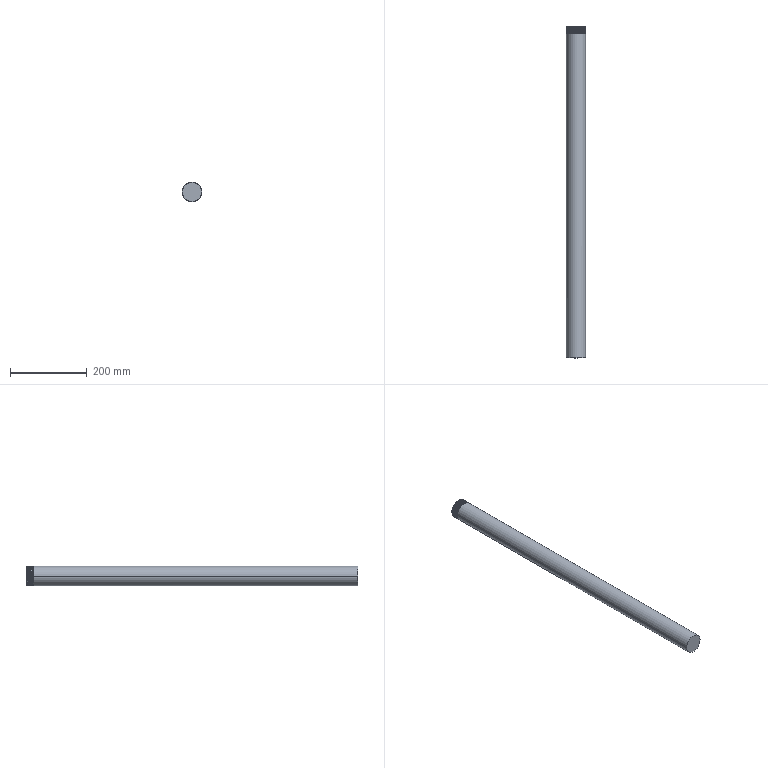Part | STEP file | Input 1 | 1 solid | 48 faces | box 50 x 864.17 x 50 mm | volume 1696768 mm3 | cylinder 42 | plane 3 | spline 3 | commonest cylinder face diameters 50 x42